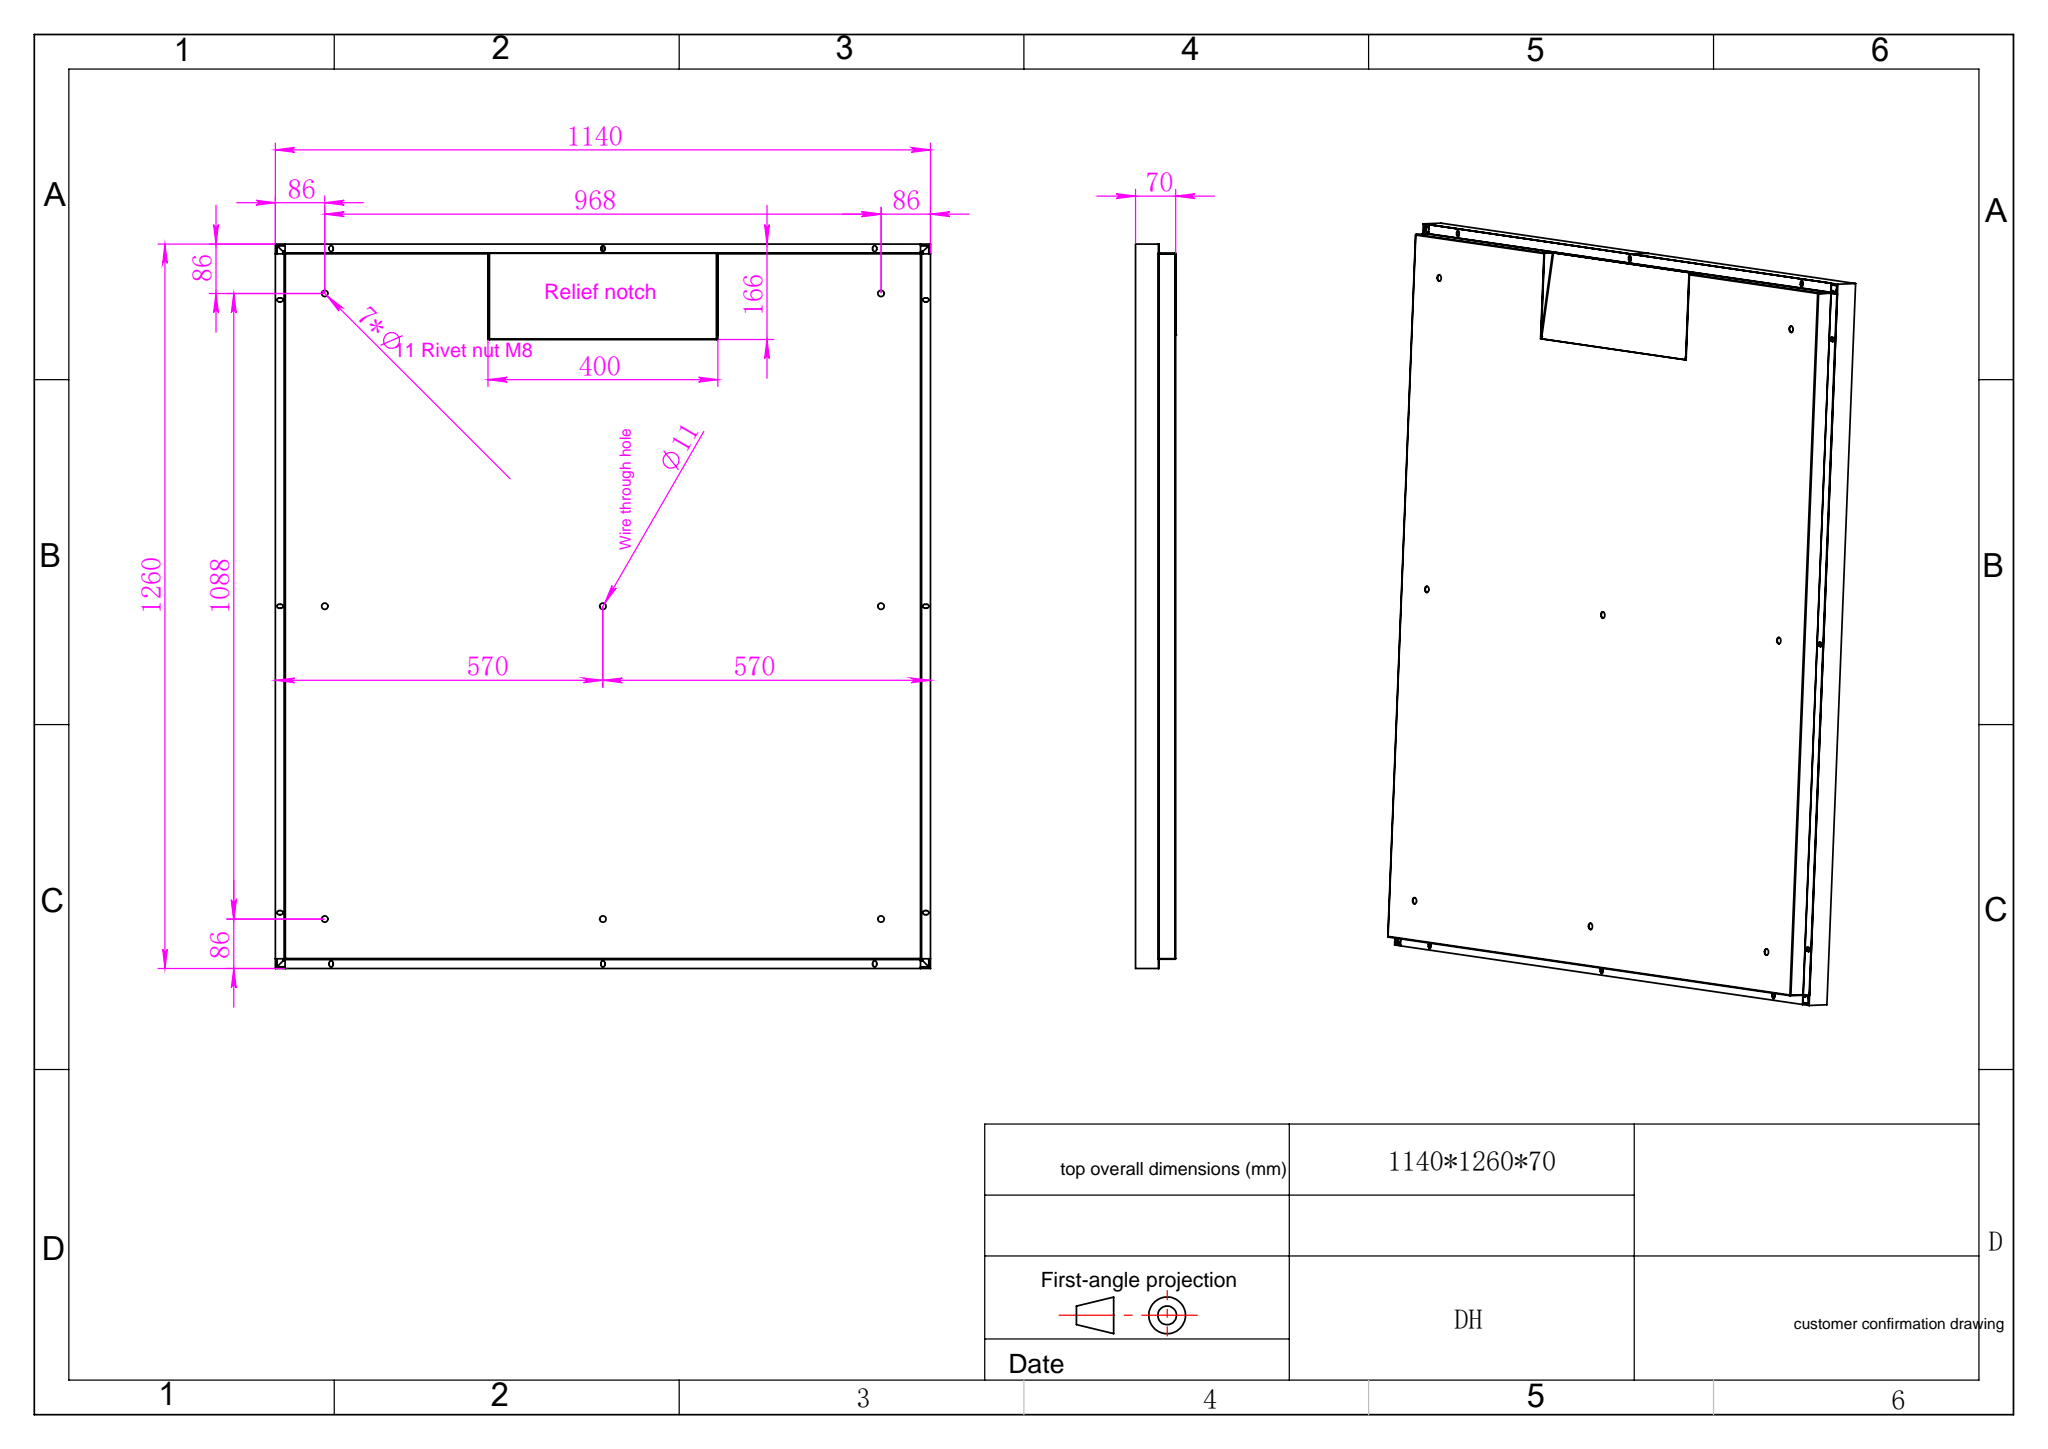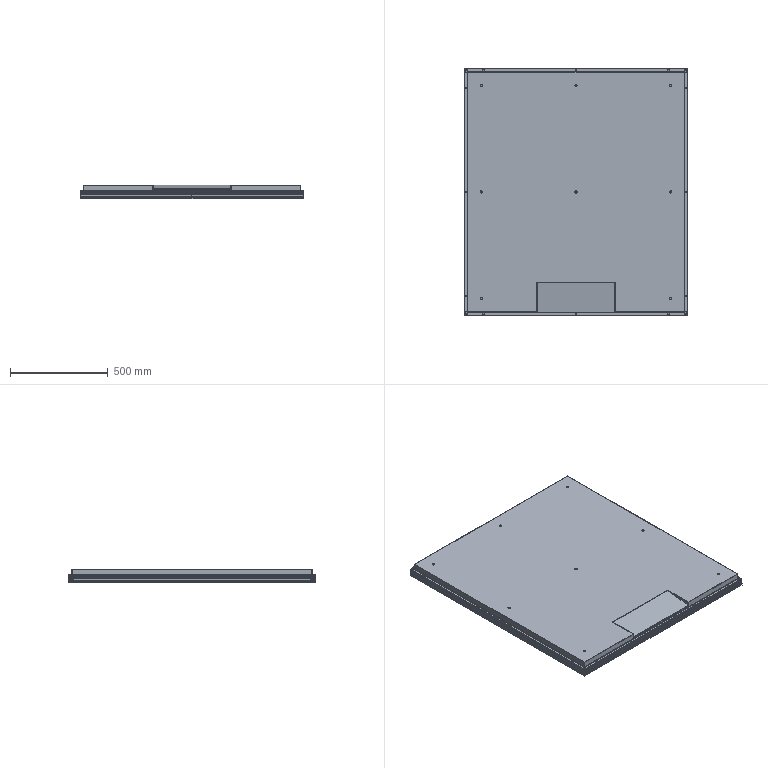Part | SolidWorks | 9 solids | 560 faces | box 1140 x 1260 x 70.147 mm | volume 18590168 mm3 | plane 344 | cylinder 204 | spline 12 | commonest cylinder face diameters 0.6 x80 4 x34 7 x30 3 x16 11 x16 0.4 x9